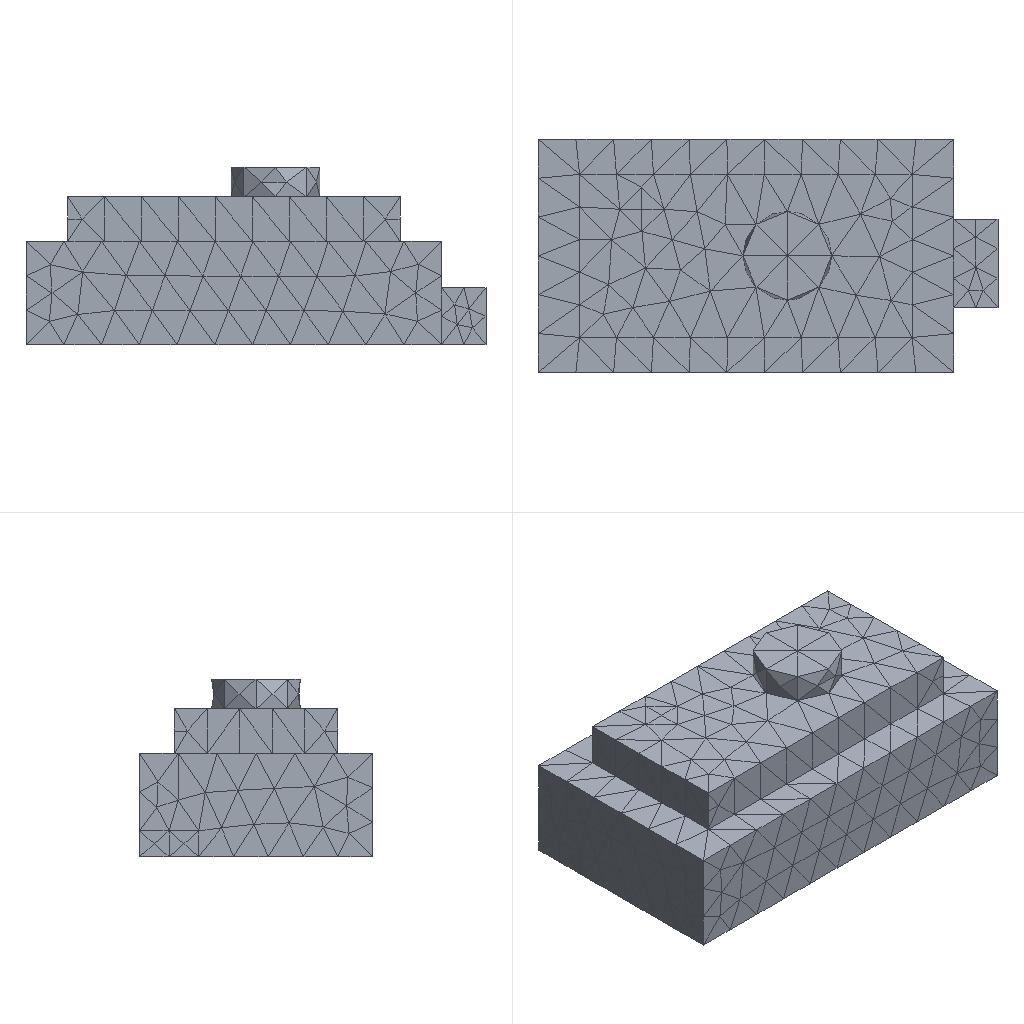Simulation study | ansys mapdl
Set-up summary:
category,name,step,type,value,unit,region
solver,ansys_mapdl
units,mm-N-s-tonne (MPa),,inferred,E=210000 density=
analysis,model,,static
mesh,nodes,,,3618
mesh,elements,,,2096
element_type,SOLID187,,,2096
material,mat 1,,E,210000
material,mat 1,,nu,0.3
load,,model,body load temp,,,all
load,,model,force,"1000 [dir=(0, 0, -1) n=291]",,node list
bc,,model,fixed,"[dofs=UX,UY,UZ n=4154]",,node list
Ansys APDL input file, long lists of numbers shortened:
/COM,ANSYS RELEASE 2026 R1           BUILD 26.1      UP20260202       09:09:58
/PREP7
/NOPR
/TITLE,2
ANTYPE, 0
*IF,_CDRDOFF,EQ,1,THEN     !if solid model was read in
_CDRDOFF=             !reset flag, numoffs already performed
*ELSE              !offset database for the following FE model
NUMOFF,NODE,     3618
NUMOFF,ELEM,     2096
NUMOFF,MAT ,        1
NUMOFF,TYPE,        1
*ENDIF
*SET,_RETURN ,  0.
*SET,_STATUS ,  0.
*SET,_UIQR   ,  291.
*SET,__FLOATPARAMETER__,  3618.
DOF,DELETE
ETBLOCK,        1,        1
(2i9,19a9)
        1      187        0        0        0        0        0        0        0        0        0        0        0        0        0        0        0        0        0        0        0
       -1
NBLOCK,6,SOLID,      3618,      3618
(3i9,6e21.13e3)
        1        0        0-4.0200000000000E+001 3.1500000000000E+001 7.0000000000000E+000
! (3617 more lines like these left out)
N,UNBL,LOC,       -1,
EBLOCK,19,SOLID,      2096,      2096
(19i10)
         1         1         1         1         0         0         0         0        10         0         1      1551       749       875       857      1730      1731      1732      1733
! (4191 more lines like these left out)
        -1
MPTEMP,UNBL, 1, 1,  0.    ,
MPDATA,UNBL, 1,EX  ,       1, 1,  210000.000    ,
MPTEMP,UNBL, 1, 1,  0.    ,
MPDATA,UNBL, 1,NUXY,       1, 1, 0.3    ,
MPTEMP,UNBL, 1, 1,  0.    ,
MPDATA,UNBL, 1,PRXY,       1, 1, 0.3    ,
EXTOPT,ATTR,      0,      0,      0
EXTOPT,ESIZE,  0,  0.
EXTOPT,ACLEAR,      0
TREF,  0.
IRLF,  0
BFUNIF,TEMP,_TINY
ACEL,  0.    ,  0.    ,  0.
OMEGA,  0.    ,  0.    ,  0.
DOMEGA,  0.    ,  0.    ,  0.
CGLOC,  0.    ,  0.    ,  0.
CGOMEGA,  0.    ,  0.    ,  0.
DCGOMG,  0.    ,  0.    ,  0.
KUSE,     0
TIME,  0.
ALPHAD,  0.
BETAD,  0.
DMPRAT,  0.
DMPSTR,  0.
CRPLIM, 0.1    ,   0
CRPLIM,  0.    ,   1
NCNV,     0, 1.000000000E+12,     0,  0.    ,  0.
NEQIT,     0
ERESX,DEFA
DBLOCK,      4154
(i9,a6,2(pg16.9))
        1  UX    0.00000000      0.00000000
! (4153 more lines like these left out)
       -1
FBLOCK,       291
(i9,a6,2(pg16.9))
      500  FZ   -3.43642612      0.00000000
! (290 more lines like these left out)
       -1
/GO
FINISH
Results summary:
result,analysis_type_db,,,static,unstated
result,n_sets,,,1,unstated
result,load_steps[0].set,load_step=1,,1,unstated
result,load_steps[0].substep,load_step=1,,1,unstated
result,load_steps[0].time,load_step=1,,1,unstated
result,load_steps[0].freq,load_step=1,,1,unstated
result,load_steps[0].max_usum,load_step=1,,9.0743e-05,unstated
result,load_steps[0].max_seqv,load_step=1,,1.269,unstated
result,load_steps[0].reaction_sum.FX,load_step=1,,-9.1247e-12,unstated
result,load_steps[0].reaction_sum.FY,load_step=1,,1.1573e-12,unstated
result,load_steps[0].reaction_sum.FZ,load_step=1,,1000,unstated
result,load_steps[0].reaction_sum.MX,load_step=1,,0,unstated
result,load_steps[0].reaction_sum.MY,load_step=1,,0,unstated
result,load_steps[0].reaction_sum.MZ,load_step=1,,0,unstated
result,convergence,,,results present for all listed sets,unstated